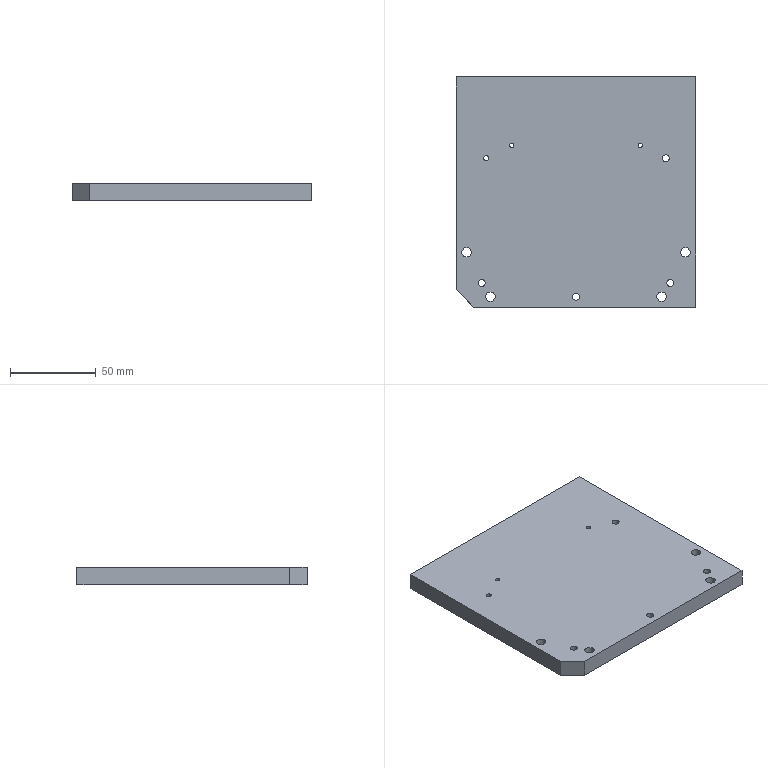Part | 1 solid | 45 faces | box 140 x 134.5 x 10 mm | volume 167544 mm3 | cylinder 23 | plane 22 | commonest cylinder face diameters 10 x10 4 x4 5.5 x4 2.5 x2 10.1 x2 3 x1
STEP:
#1=CARTESIAN_POINT('',(35.,62.25,7.));
#2=VERTEX_POINT('',#1);
#3=CARTESIAN_POINT('',(30.,57.25,7.));
#4=VERTEX_POINT('',#3);
#5=CARTESIAN_POINT('',(30.,62.25,7.));
#6=DIRECTION('',(0.,0.,-1.));
#7=DIRECTION('',(1.,0.,0.));
#8=AXIS2_PLACEMENT_3D('',#5,#6,#7);
#9=CIRCLE('',#8,5.);
#10=EDGE_CURVE('',#2,#4,#9,.T.);
#11=ORIENTED_EDGE('',*,*,#10,.F.);
#12=CARTESIAN_POINT('',(35.,62.25,0.));
#13=VERTEX_POINT('',#12);
#14=CARTESIAN_POINT('',(35.,62.25,7.));
#15=DIRECTION('',(0.,0.,1.));
#16=VECTOR('',#15,1000.);
#17=LINE('',#14,#16);
#18=EDGE_CURVE('',#13,#2,#17,.T.);
#19=ORIENTED_EDGE('',*,*,#18,.F.);
#20=CARTESIAN_POINT('',(30.,57.25,0.));
#21=VERTEX_POINT('',#20);
#22=CARTESIAN_POINT('',(30.,62.25,0.));
#23=DIRECTION('',(0.,0.,1.));
#24=DIRECTION('',(1.,0.,0.));
#25=AXIS2_PLACEMENT_3D('',#22,#23,#24);
#26=CIRCLE('',#25,5.);
#27=EDGE_CURVE('',#21,#13,#26,.T.);
#28=ORIENTED_EDGE('',*,*,#27,.F.);
#29=CARTESIAN_POINT('',(30.,57.25,0.));
#30=DIRECTION('',(0.,0.,-1.));
#31=VECTOR('',#30,1000.);
#32=LINE('',#29,#31);
#33=EDGE_CURVE('',#4,#21,#32,.T.);
#34=ORIENTED_EDGE('',*,*,#33,.F.);
#35=EDGE_LOOP('',(#11,#19,#28,#34));
#36=FACE_BOUND('',#35,.T.);
#37=CARTESIAN_POINT('',(30.,62.25,7.));
#38=DIRECTION('',(0.,0.,1.));
#39=DIRECTION('',(1.,0.,0.));
#40=AXIS2_PLACEMENT_3D('',#37,#38,#39);
#41=CYLINDRICAL_SURFACE('',#40,5.);
#42=ADVANCED_FACE('',(#36),#41,.F.);
#43=CARTESIAN_POINT('',(-30.,57.25,7.));
#44=VERTEX_POINT('',#43);
#45=CARTESIAN_POINT('',(-35.,62.25,7.));
#46=VERTEX_POINT('',#45);
#47=CARTESIAN_POINT('',(-30.,62.25,7.));
#48=DIRECTION('',(0.,0.,-1.));
#49=DIRECTION('',(1.,0.,0.));
#50=AXIS2_PLACEMENT_3D('',#47,#48,#49);
#51=CIRCLE('',#50,5.);
#52=EDGE_CURVE('',#44,#46,#51,.T.);
#53=ORIENTED_EDGE('',*,*,#52,.F.);
#54=CARTESIAN_POINT('',(-30.,57.25,0.));
#55=VERTEX_POINT('',#54);
#56=CARTESIAN_POINT('',(-30.,57.25,7.));
#57=DIRECTION('',(0.,0.,1.));
#58=VECTOR('',#57,1000.);
#59=LINE('',#56,#58);
#60=EDGE_CURVE('',#55,#44,#59,.T.);
#61=ORIENTED_EDGE('',*,*,#60,.F.);
#62=CARTESIAN_POINT('',(-35.,62.25,0.));
#63=VERTEX_POINT('',#62);
#64=CARTESIAN_POINT('',(-30.,62.25,0.));
#65=DIRECTION('',(0.,0.,1.));
#66=DIRECTION('',(1.,0.,0.));
#67=AXIS2_PLACEMENT_3D('',#64,#65,#66);
#68=CIRCLE('',#67,5.);
#69=EDGE_CURVE('',#63,#55,#68,.T.);
#70=ORIENTED_EDGE('',*,*,#69,.F.);
#71=CARTESIAN_POINT('',(-35.,62.25,7.));
#72=DIRECTION('',(0.,0.,-1.));
#73=VECTOR('',#72,1000.);
#74=LINE('',#71,#73);
#75=EDGE_CURVE('',#46,#63,#74,.T.);
#76=ORIENTED_EDGE('',*,*,#75,.F.);
#77=EDGE_LOOP('',(#53,#61,#70,#76));
#78=FACE_BOUND('',#77,.T.);
#79=CARTESIAN_POINT('',(-30.,62.25,7.));
#80=DIRECTION('',(0.,0.,1.));
#81=DIRECTION('',(1.,0.,0.));
#82=AXIS2_PLACEMENT_3D('',#79,#80,#81);
#83=CYLINDRICAL_SURFACE('',#82,5.);
#84=ADVANCED_FACE('',(#78),#83,.F.);
#85=CARTESIAN_POINT('',(30.,-7.75,7.));
#86=VERTEX_POINT('',#85);
#87=CARTESIAN_POINT('',(35.,-12.75,7.));
#88=VERTEX_POINT('',#87);
#89=CARTESIAN_POINT('',(30.,-12.75,7.));
#90=DIRECTION('',(0.,0.,-1.));
#91=DIRECTION('',(1.,0.,0.));
#92=AXIS2_PLACEMENT_3D('',#89,#90,#91);
#93=CIRCLE('',#92,5.);
#94=EDGE_CURVE('',#86,#88,#93,.T.);
#95=ORIENTED_EDGE('',*,*,#94,.F.);
#96=CARTESIAN_POINT('',(30.,-7.75,0.));
#97=VERTEX_POINT('',#96);
#98=CARTESIAN_POINT('',(30.,-7.75,7.));
#99=DIRECTION('',(0.,0.,1.));
#100=VECTOR('',#99,1000.);
#101=LINE('',#98,#100);
#102=EDGE_CURVE('',#97,#86,#101,.T.);
#103=ORIENTED_EDGE('',*,*,#102,.F.);
#104=CARTESIAN_POINT('',(35.,-12.75,0.));
#105=VERTEX_POINT('',#104);
#106=CARTESIAN_POINT('',(30.,-12.75,0.));
#107=DIRECTION('',(0.,0.,1.));
#108=DIRECTION('',(1.,0.,0.));
#109=AXIS2_PLACEMENT_3D('',#106,#107,#108);
#110=CIRCLE('',#109,5.);
#111=EDGE_CURVE('',#105,#97,#110,.T.);
#112=ORIENTED_EDGE('',*,*,#111,.F.);
#113=CARTESIAN_POINT('',(35.,-12.75,0.));
#114=DIRECTION('',(0.,0.,-1.));
#115=VECTOR('',#114,1000.);
#116=LINE('',#113,#115);
#117=EDGE_CURVE('',#88,#105,#116,.T.);
#118=ORIENTED_EDGE('',*,*,#117,.F.);
#119=EDGE_LOOP('',(#95,#103,#112,#118));
#120=FACE_BOUND('',#119,.T.);
#121=CARTESIAN_POINT('',(30.,-12.75,7.));
#122=DIRECTION('',(0.,0.,1.));
#123=DIRECTION('',(1.,0.,0.));
#124=AXIS2_PLACEMENT_3D('',#121,#122,#123);
#125=CYLINDRICAL_SURFACE('',#124,5.);
#126=ADVANCED_FACE('',(#120),#125,.F.);
#127=CARTESIAN_POINT('',(35.,-27.75,7.));
#128=VERTEX_POINT('',#127);
#129=CARTESIAN_POINT('',(30.,-32.75,7.));
#130=VERTEX_POINT('',#129);
#131=CARTESIAN_POINT('',(30.,-27.75,7.));
#132=DIRECTION('',(0.,0.,-1.));
#133=DIRECTION('',(1.,0.,0.));
#134=AXIS2_PLACEMENT_3D('',#131,#132,#133);
#135=CIRCLE('',#134,5.);
#136=EDGE_CURVE('',#128,#130,#135,.T.);
#137=ORIENTED_EDGE('',*,*,#136,.F.);
#138=CARTESIAN_POINT('',(35.,-27.75,0.));
#139=VERTEX_POINT('',#138);
#140=CARTESIAN_POINT('',(35.,-27.75,7.));
#141=DIRECTION('',(0.,0.,1.));
#142=VECTOR('',#141,1000.);
#143=LINE('',#140,#142);
#144=EDGE_CURVE('',#139,#128,#143,.T.);
#145=ORIENTED_EDGE('',*,*,#144,.F.);
#146=CARTESIAN_POINT('',(30.,-32.75,0.));
#147=VERTEX_POINT('',#146);
#148=CARTESIAN_POINT('',(30.,-27.75,0.));
#149=DIRECTION('',(0.,0.,1.));
#150=DIRECTION('',(1.,0.,0.));
#151=AXIS2_PLACEMENT_3D('',#148,#149,#150);
#152=CIRCLE('',#151,5.);
#153=EDGE_CURVE('',#147,#139,#152,.T.);
#154=ORIENTED_EDGE('',*,*,#153,.F.);
#155=CARTESIAN_POINT('',(30.,-32.75,0.));
#156=DIRECTION('',(0.,0.,-1.));
#157=VECTOR('',#156,1000.);
#158=LINE('',#155,#157);
#159=EDGE_CURVE('',#130,#147,#158,.T.);
#160=ORIENTED_EDGE('',*,*,#159,.F.);
#161=EDGE_LOOP('',(#137,#145,#154,#160));
#162=FACE_BOUND('',#161,.T.);
#163=CARTESIAN_POINT('',(30.,-27.75,7.));
#164=DIRECTION('',(0.,0.,1.));
#165=DIRECTION('',(1.,0.,0.));
#166=AXIS2_PLACEMENT_3D('',#163,#164,#165);
#167=CYLINDRICAL_SURFACE('',#166,5.);
#168=ADVANCED_FACE('',(#162),#167,.F.);
#169=CARTESIAN_POINT('',(-35.,-12.75,7.));
#170=VERTEX_POINT('',#169);
#171=CARTESIAN_POINT('',(-30.,-7.75,7.));
#172=VERTEX_POINT('',#171);
#173=CARTESIAN_POINT('',(-30.,-12.75,7.));
#174=DIRECTION('',(0.,0.,-1.));
#175=DIRECTION('',(1.,0.,0.));
#176=AXIS2_PLACEMENT_3D('',#173,#174,#175);
#177=CIRCLE('',#176,5.);
#178=EDGE_CURVE('',#170,#172,#177,.T.);
#179=ORIENTED_EDGE('',*,*,#178,.F.);
#180=CARTESIAN_POINT('',(-35.,-12.75,0.));
#181=VERTEX_POINT('',#180);
#182=CARTESIAN_POINT('',(-35.,-12.75,7.));
#183=DIRECTION('',(0.,0.,1.));
#184=VECTOR('',#183,1000.);
#185=LINE('',#182,#184);
#186=EDGE_CURVE('',#181,#170,#185,.T.);
#187=ORIENTED_EDGE('',*,*,#186,.F.);
#188=CARTESIAN_POINT('',(-30.,-7.75,0.));
#189=VERTEX_POINT('',#188);
#190=CARTESIAN_POINT('',(-30.,-12.75,0.));
#191=DIRECTION('',(0.,0.,1.));
#192=DIRECTION('',(1.,0.,0.));
#193=AXIS2_PLACEMENT_3D('',#190,#191,#192);
#194=CIRCLE('',#193,5.);
#195=EDGE_CURVE('',#189,#181,#194,.T.);
#196=ORIENTED_EDGE('',*,*,#195,.F.);
#197=CARTESIAN_POINT('',(-30.,-7.75,0.));
#198=DIRECTION('',(0.,0.,-1.));
#199=VECTOR('',#198,1000.);
#200=LINE('',#197,#199);
#201=EDGE_CURVE('',#172,#189,#200,.T.);
#202=ORIENTED_EDGE('',*,*,#201,.F.);
#203=EDGE_LOOP('',(#179,#187,#196,#202));
#204=FACE_BOUND('',#203,.T.);
#205=CARTESIAN_POINT('',(-30.,-12.75,7.));
#206=DIRECTION('',(0.,0.,1.));
#207=DIRECTION('',(1.,0.,0.));
#208=AXIS2_PLACEMENT_3D('',#205,#206,#207);
#209=CYLINDRICAL_SURFACE('',#208,5.);
#210=ADVANCED_FACE('',(#204),#209,.F.);
#211=CARTESIAN_POINT('',(-30.,-32.75,7.));
#212=VERTEX_POINT('',#211);
#213=CARTESIAN_POINT('',(-35.,-27.75,7.));
#214=VERTEX_POINT('',#213);
#215=CARTESIAN_POINT('',(-30.,-27.75,7.));
#216=DIRECTION('',(0.,0.,-1.));
#217=DIRECTION('',(1.,0.,0.));
#218=AXIS2_PLACEMENT_3D('',#215,#216,#217);
#219=CIRCLE('',#218,5.);
#220=EDGE_CURVE('',#212,#214,#219,.T.);
#221=ORIENTED_EDGE('',*,*,#220,.F.);
#222=CARTESIAN_POINT('',(-30.,-32.75,0.));
#223=VERTEX_POINT('',#222);
#224=CARTESIAN_POINT('',(-30.,-32.75,7.));
#225=DIRECTION('',(0.,0.,1.));
#226=VECTOR('',#225,1000.);
#227=LINE('',#224,#226);
#228=EDGE_CURVE('',#223,#212,#227,.T.);
#229=ORIENTED_EDGE('',*,*,#228,.F.);
#230=CARTESIAN_POINT('',(-35.,-27.75,0.));
#231=VERTEX_POINT('',#230);
#232=CARTESIAN_POINT('',(-30.,-27.75,0.));
#233=DIRECTION('',(0.,0.,1.));
#234=DIRECTION('',(1.,0.,0.));
#235=AXIS2_PLACEMENT_3D('',#232,#233,#234);
#236=CIRCLE('',#235,5.);
#237=EDGE_CURVE('',#231,#223,#236,.T.);
#238=ORIENTED_EDGE('',*,*,#237,.F.);
#239=CARTESIAN_POINT('',(-35.,-27.75,0.));
#240=DIRECTION('',(0.,0.,-1.));
#241=VECTOR('',#240,1000.);
#242=LINE('',#239,#241);
#243=EDGE_CURVE('',#214,#231,#242,.T.);
#244=ORIENTED_EDGE('',*,*,#243,.F.);
#245=EDGE_LOOP('',(#221,#229,#238,#244));
#246=FACE_BOUND('',#245,.T.);
#247=CARTESIAN_POINT('',(-30.,-27.75,7.));
#248=DIRECTION('',(0.,0.,1.));
#249=DIRECTION('',(1.,0.,0.));
#250=AXIS2_PLACEMENT_3D('',#247,#248,#249);
#251=CYLINDRICAL_SURFACE('',#250,5.);
#252=ADVANCED_FACE('',(#246),#251,.F.);
#253=CARTESIAN_POINT('',(35.,-32.75,7.));
#254=DIRECTION('',(-1.,0.,0.));
#255=VECTOR('',#254,1000.);
#256=LINE('',#253,#255);
#257=EDGE_CURVE('',#130,#212,#256,.T.);
#258=ORIENTED_EDGE('',*,*,#257,.T.);
#259=ORIENTED_EDGE('',*,*,#220,.T.);
#260=CARTESIAN_POINT('',(-35.,-32.75,7.));
#261=DIRECTION('',(0.,1.,0.));
#262=VECTOR('',#261,1000.);
#263=LINE('',#260,#262);
#264=EDGE_CURVE('',#214,#170,#263,.T.);
#265=ORIENTED_EDGE('',*,*,#264,.T.);
#266=ORIENTED_EDGE('',*,*,#178,.T.);
#267=CARTESIAN_POINT('',(35.,-7.75,7.));
#268=DIRECTION('',(1.,0.,0.));
#269=VECTOR('',#268,1000.);
#270=LINE('',#267,#269);
#271=EDGE_CURVE('',#172,#86,#270,.T.);
#272=ORIENTED_EDGE('',*,*,#271,.T.);
#273=ORIENTED_EDGE('',*,*,#94,.T.);
#274=CARTESIAN_POINT('',(35.,-32.75,7.));
#275=DIRECTION('',(0.,-1.,0.));
#276=VECTOR('',#275,1000.);
#277=LINE('',#274,#276);
#278=EDGE_CURVE('',#88,#128,#277,.T.);
#279=ORIENTED_EDGE('',*,*,#278,.T.);
#280=ORIENTED_EDGE('',*,*,#136,.T.);
#281=EDGE_LOOP('',(#258,#259,#265,#266,#272,#273,#279,#280));
#282=FACE_BOUND('',#281,.T.);
#283=CARTESIAN_POINT('',(0.,0.,7.));
#284=DIRECTION('',(0.,0.,1.));
#285=DIRECTION('',(1.,0.,0.));
#286=AXIS2_PLACEMENT_3D('',#283,#284,#285);
#287=PLANE('',#286);
#288=ADVANCED_FACE('',(#282),#287,.F.);
#289=CARTESIAN_POINT('',(35.,-32.75,0.));
#290=DIRECTION('',(-1.,0.,0.));
#291=VECTOR('',#290,1000.);
#292=LINE('',#289,#291);
#293=EDGE_CURVE('',#147,#223,#292,.T.);
#294=ORIENTED_EDGE('',*,*,#293,.T.);
#295=ORIENTED_EDGE('',*,*,#228,.T.);
#296=ORIENTED_EDGE('',*,*,#257,.F.);
#297=ORIENTED_EDGE('',*,*,#159,.T.);
#298=EDGE_LOOP('',(#294,#295,#296,#297));
#299=FACE_BOUND('',#298,.T.);
#300=CARTESIAN_POINT('',(35.,-32.75,7.));
#301=DIRECTION('',(0.,-1.,0.));
#302=DIRECTION('',(0.,0.,-1.));
#303=AXIS2_PLACEMENT_3D('',#300,#301,#302);
#304=PLANE('',#303);
#305=ADVANCED_FACE('',(#299),#304,.F.);
#306=ORIENTED_EDGE('',*,*,#264,.F.);
#307=ORIENTED_EDGE('',*,*,#243,.T.);
#308=CARTESIAN_POINT('',(-35.,-32.75,0.));
#309=DIRECTION('',(0.,1.,0.));
#310=VECTOR('',#309,1000.);
#311=LINE('',#308,#310);
#312=EDGE_CURVE('',#231,#181,#311,.T.);
#313=ORIENTED_EDGE('',*,*,#312,.T.);
#314=ORIENTED_EDGE('',*,*,#186,.T.);
#315=EDGE_LOOP('',(#306,#307,#313,#314));
#316=FACE_BOUND('',#315,.T.);
#317=CARTESIAN_POINT('',(-35.,-32.75,7.));
#318=DIRECTION('',(-1.,0.,0.));
#319=DIRECTION('',(0.,0.,1.));
#320=AXIS2_PLACEMENT_3D('',#317,#318,#319);
#321=PLANE('',#320);
#322=ADVANCED_FACE('',(#316),#321,.F.);
#323=ORIENTED_EDGE('',*,*,#271,.F.);
#324=ORIENTED_EDGE('',*,*,#201,.T.);
#325=CARTESIAN_POINT('',(35.,-7.75,0.));
#326=DIRECTION('',(1.,0.,0.));
#327=VECTOR('',#326,1000.);
#328=LINE('',#325,#327);
#329=EDGE_CURVE('',#189,#97,#328,.T.);
#330=ORIENTED_EDGE('',*,*,#329,.T.);
#331=ORIENTED_EDGE('',*,*,#102,.T.);
#332=EDGE_LOOP('',(#323,#324,#330,#331));
#333=FACE_BOUND('',#332,.T.);
#334=CARTESIAN_POINT('',(35.,-7.75,7.));
#335=DIRECTION('',(0.,1.,0.));
#336=DIRECTION('',(0.,0.,1.));
#337=AXIS2_PLACEMENT_3D('',#334,#335,#336);
#338=PLANE('',#337);
#339=ADVANCED_FACE('',(#333),#338,.F.);
#340=CARTESIAN_POINT('',(35.,-32.75,0.));
#341=DIRECTION('',(0.,-1.,0.));
#342=VECTOR('',#341,1000.);
#343=LINE('',#340,#342);
#344=EDGE_CURVE('',#105,#139,#343,.T.);
#345=ORIENTED_EDGE('',*,*,#344,.T.);
#346=ORIENTED_EDGE('',*,*,#144,.T.);
#347=ORIENTED_EDGE('',*,*,#278,.F.);
#348=ORIENTED_EDGE('',*,*,#117,.T.);
#349=EDGE_LOOP('',(#345,#346,#347,#348));
#350=FACE_BOUND('',#349,.T.);
#351=CARTESIAN_POINT('',(35.,-32.75,7.));
#352=DIRECTION('',(1.,0.,0.));
#353=DIRECTION('',(0.,0.,-1.));
#354=AXIS2_PLACEMENT_3D('',#351,#352,#353);
#355=PLANE('',#354);
#356=ADVANCED_FACE('',(#350),#355,.F.);
#357=CARTESIAN_POINT('',(-35.,57.25,7.));
#358=DIRECTION('',(-1.,0.,0.));
#359=VECTOR('',#358,1000.);
#360=LINE('',#357,#359);
#361=EDGE_CURVE('',#4,#44,#360,.T.);
#362=ORIENTED_EDGE('',*,*,#361,.T.);
#363=ORIENTED_EDGE('',*,*,#52,.T.);
#364=CARTESIAN_POINT('',(-35.,67.25,7.));
#365=VERTEX_POINT('',#364);
#366=CARTESIAN_POINT('',(-35.,0.,7.));
#367=DIRECTION('',(0.,1.,0.));
#368=VECTOR('',#367,1000.);
#369=LINE('',#366,#368);
#370=EDGE_CURVE('',#46,#365,#369,.T.);
#371=ORIENTED_EDGE('',*,*,#370,.T.);
#372=CARTESIAN_POINT('',(35.,67.25,7.));
#373=VERTEX_POINT('',#372);
#374=CARTESIAN_POINT('',(-35.,67.25,7.));
#375=DIRECTION('',(1.,0.,0.));
#376=VECTOR('',#375,1000.);
#377=LINE('',#374,#376);
#378=EDGE_CURVE('',#365,#373,#377,.T.);
#379=ORIENTED_EDGE('',*,*,#378,.T.);
#380=CARTESIAN_POINT('',(35.,0.,7.));
#381=DIRECTION('',(0.,-1.,0.));
#382=VECTOR('',#381,1000.);
#383=LINE('',#380,#382);
#384=EDGE_CURVE('',#373,#2,#383,.T.);
#385=ORIENTED_EDGE('',*,*,#384,.T.);
#386=ORIENTED_EDGE('',*,*,#10,.T.);
#387=EDGE_LOOP('',(#362,#363,#371,#379,#385,#386));
#388=FACE_BOUND('',#387,.T.);
#389=CARTESIAN_POINT('',(0.,0.,7.));
#390=DIRECTION('',(0.,0.,1.));
#391=DIRECTION('',(1.,0.,0.));
#392=AXIS2_PLACEMENT_3D('',#389,#390,#391);
#393=PLANE('',#392);
#394=ADVANCED_FACE('',(#388),#393,.F.);
#395=CARTESIAN_POINT('',(35.,67.25,0.));
#396=VERTEX_POINT('',#395);
#397=CARTESIAN_POINT('',(35.,-32.75,0.));
#398=DIRECTION('',(0.,-1.,0.));
#399=VECTOR('',#398,1000.);
#400=LINE('',#397,#399);
#401=EDGE_CURVE('',#396,#13,#400,.T.);
#402=ORIENTED_EDGE('',*,*,#401,.T.);
#403=ORIENTED_EDGE('',*,*,#18,.T.);
#404=ORIENTED_EDGE('',*,*,#384,.F.);
#405=CARTESIAN_POINT('',(35.,67.25,7.));
#406=DIRECTION('',(0.,0.,-1.));
#407=VECTOR('',#406,1000.);
#408=LINE('',#405,#407);
#409=EDGE_CURVE('',#373,#396,#408,.T.);
#410=ORIENTED_EDGE('',*,*,#409,.T.);
#411=EDGE_LOOP('',(#402,#403,#404,#410));
#412=FACE_BOUND('',#411,.T.);
#413=CARTESIAN_POINT('',(35.,-32.75,7.));
#414=DIRECTION('',(1.,0.,0.));
#415=DIRECTION('',(0.,0.,-1.));
#416=AXIS2_PLACEMENT_3D('',#413,#414,#415);
#417=PLANE('',#416);
#418=ADVANCED_FACE('',(#412),#417,.F.);
#419=CARTESIAN_POINT('',(-35.,57.25,0.));
#420=DIRECTION('',(-1.,0.,0.));
#421=VECTOR('',#420,1000.);
#422=LINE('',#419,#421);
#423=EDGE_CURVE('',#21,#55,#422,.T.);
#424=ORIENTED_EDGE('',*,*,#423,.T.);
#425=ORIENTED_EDGE('',*,*,#60,.T.);
#426=ORIENTED_EDGE('',*,*,#361,.F.);
#427=ORIENTED_EDGE('',*,*,#33,.T.);
#428=EDGE_LOOP('',(#424,#425,#426,#427));
#429=FACE_BOUND('',#428,.T.);
#430=CARTESIAN_POINT('',(-35.,57.25,7.));
#431=DIRECTION('',(0.,-1.,0.));
#432=DIRECTION('',(0.,0.,-1.));
#433=AXIS2_PLACEMENT_3D('',#430,#431,#432);
#434=PLANE('',#433);
#435=ADVANCED_FACE('',(#429),#434,.F.);
#436=ORIENTED_EDGE('',*,*,#370,.F.);
#437=ORIENTED_EDGE('',*,*,#75,.T.);
#438=CARTESIAN_POINT('',(-35.,67.25,0.));
#439=VERTEX_POINT('',#438);
#440=CARTESIAN_POINT('',(-35.,-32.75,0.));
#441=DIRECTION('',(0.,1.,0.));
#442=VECTOR('',#441,1000.);
#443=LINE('',#440,#442);
#444=EDGE_CURVE('',#63,#439,#443,.T.);
#445=ORIENTED_EDGE('',*,*,#444,.T.);
#446=CARTESIAN_POINT('',(-35.,67.25,10.));
#447=DIRECTION('',(0.,0.,-1.));
#448=VECTOR('',#447,1000.);
#449=LINE('',#446,#448);
#450=EDGE_CURVE('',#365,#439,#449,.T.);
#451=ORIENTED_EDGE('',*,*,#450,.F.);
#452=EDGE_LOOP('',(#436,#437,#445,#451));
#453=FACE_BOUND('',#452,.T.);
#454=CARTESIAN_POINT('',(-35.,-32.75,7.));
#455=DIRECTION('',(-1.,0.,0.));
#456=DIRECTION('',(0.,0.,1.));
#457=AXIS2_PLACEMENT_3D('',#454,#455,#456);
#458=PLANE('',#457);
#459=ADVANCED_FACE('',(#453),#458,.F.);
#460=CARTESIAN_POINT('',(32.45,27.25,3.5));
#461=VERTEX_POINT('',#460);
#462=CARTESIAN_POINT('',(37.5,27.25,3.5));
#463=DIRECTION('',(0.,0.,-1.));
#464=DIRECTION('',(-1.,0.,0.));
#465=AXIS2_PLACEMENT_3D('',#462,#463,#464);
#466=CIRCLE('',#465,5.05);
#467=EDGE_CURVE('',#461,#461,#466,.T.);
#468=ORIENTED_EDGE('',*,*,#467,.T.);
#469=EDGE_LOOP('',(#468));
#470=FACE_BOUND('',#469,.T.);
#471=CARTESIAN_POINT('',(36.25,27.25,3.5));
#472=VERTEX_POINT('',#471);
#473=CARTESIAN_POINT('',(37.5,27.25,3.5));
#474=DIRECTION('',(0.,0.,-1.));
#475=DIRECTION('',(-1.,0.,0.));
#476=AXIS2_PLACEMENT_3D('',#473,#474,#475);
#477=CIRCLE('',#476,1.25);
#478=EDGE_CURVE('',#472,#472,#477,.T.);
#479=ORIENTED_EDGE('',*,*,#478,.F.);
#480=EDGE_LOOP('',(#479));
#481=FACE_BOUND('',#480,.T.);
#482=CARTESIAN_POINT('',(37.5,27.25,3.5));
#483=DIRECTION('',(0.,0.,1.));
#484=DIRECTION('',(1.,0.,0.));
#485=AXIS2_PLACEMENT_3D('',#482,#483,#484);
#486=PLANE('',#485);
#487=ADVANCED_FACE('',(#470,#481),#486,.F.);
#488=CARTESIAN_POINT('',(-32.45,27.25,3.5));
#489=VERTEX_POINT('',#488);
#490=CARTESIAN_POINT('',(-37.5,27.25,3.5));
#491=DIRECTION('',(0.,0.,-1.));
#492=DIRECTION('',(1.,0.,0.));
#493=AXIS2_PLACEMENT_3D('',#490,#491,#492);
#494=CIRCLE('',#493,5.05);
#495=EDGE_CURVE('',#489,#489,#494,.T.);
#496=ORIENTED_EDGE('',*,*,#495,.T.);
#497=EDGE_LOOP('',(#496));
#498=FACE_BOUND('',#497,.T.);
#499=CARTESIAN_POINT('',(-36.25,27.25,3.5));
#500=VERTEX_POINT('',#499);
#501=CARTESIAN_POINT('',(-37.5,27.25,3.5));
#502=DIRECTION('',(0.,0.,-1.));
#503=DIRECTION('',(1.,0.,0.));
#504=AXIS2_PLACEMENT_3D('',#501,#502,#503);
#505=CIRCLE('',#504,1.25);
#506=EDGE_CURVE('',#500,#500,#505,.T.);
#507=ORIENTED_EDGE('',*,*,#506,.F.);
#508=EDGE_LOOP('',(#507));
#509=FACE_BOUND('',#508,.T.);
#510=CARTESIAN_POINT('',(37.5,27.25,3.5));
#511=DIRECTION('',(0.,0.,1.));
#512=DIRECTION('',(1.,0.,0.));
#513=AXIS2_PLACEMENT_3D('',#510,#511,#512);
#514=PLANE('',#513);
#515=ADVANCED_FACE('',(#498,#509),#514,.F.);
#516=CARTESIAN_POINT('',(-70.,-57.25,10.));
#517=VERTEX_POINT('',#516);
#518=CARTESIAN_POINT('',(-60.,-67.25,10.));
#519=VERTEX_POINT('',#518);
#520=CARTESIAN_POINT('',(-63.625,-63.625,10.));
#521=DIRECTION('',(0.7071,-0.7071,0.));
#522=VECTOR('',#521,1000.);
#523=LINE('',#520,#522);
#524=EDGE_CURVE('',#517,#519,#523,.T.);
#525=ORIENTED_EDGE('',*,*,#524,.F.);
#526=CARTESIAN_POINT('',(-70.,-57.25,0.));
#527=VERTEX_POINT('',#526);
#528=CARTESIAN_POINT('',(-70.,-57.25,10.));
#529=DIRECTION('',(0.,0.,1.));
#530=VECTOR('',#529,1000.);
#531=LINE('',#528,#530);
#532=EDGE_CURVE('',#527,#517,#531,.T.);
#533=ORIENTED_EDGE('',*,*,#532,.F.);
#534=CARTESIAN_POINT('',(-60.,-67.25,0.));
#535=VERTEX_POINT('',#534);
#536=CARTESIAN_POINT('',(-60.,-67.25,0.));
#537=DIRECTION('',(-0.7071,0.7071,0.));
#538=VECTOR('',#537,1000.);
#539=LINE('',#536,#538);
#540=EDGE_CURVE('',#535,#527,#539,.T.);
#541=ORIENTED_EDGE('',*,*,#540,.F.);
#542=CARTESIAN_POINT('',(-60.,-67.25,10.));
#543=DIRECTION('',(0.,0.,-1.));
#544=VECTOR('',#543,1000.);
#545=LINE('',#542,#544);
#546=EDGE_CURVE('',#519,#535,#545,.T.);
#547=ORIENTED_EDGE('',*,*,#546,.F.);
#548=EDGE_LOOP('',(#525,#533,#541,#547));
#549=FACE_BOUND('',#548,.T.);
#550=CARTESIAN_POINT('',(-60.,-67.25,10.));
#551=DIRECTION('',(0.7071,0.7071,0.));
#552=DIRECTION('',(0.,0.,-1.));
#553=AXIS2_PLACEMENT_3D('',#550,#551,#552);
#554=PLANE('',#553);
#555=ADVANCED_FACE('',(#549),#554,.F.);
#556=CARTESIAN_POINT('',(45.,-61.25,5.4));
#557=VERTEX_POINT('',#556);
#558=CARTESIAN_POINT('',(50.,-61.25,5.4));
#559=DIRECTION('',(0.,0.,-1.));
#560=DIRECTION('',(-1.,0.,0.));
#561=AXIS2_PLACEMENT_3D('',#558,#559,#560);
#562=CIRCLE('',#561,5.);
#563=EDGE_CURVE('',#557,#557,#562,.T.);
#564=ORIENTED_EDGE('',*,*,#563,.T.);
#565=EDGE_LOOP('',(#564));
#566=FACE_BOUND('',#565,.T.);
#567=CARTESIAN_POINT('',(47.25,-61.25,5.4));
#568=VERTEX_POINT('',#567);
#569=CARTESIAN_POINT('',(50.,-61.25,5.4));
#570=DIRECTION('',(0.,0.,-1.));
#571=DIRECTION('',(-1.,0.,0.));
#572=AXIS2_PLACEMENT_3D('',#569,#570,#571);
#573=CIRCLE('',#572,2.75);
#574=EDGE_CURVE('',#568,#568,#573,.T.);
#575=ORIENTED_EDGE('',*,*,#574,.F.);
#576=EDGE_LOOP('',(#575));
#577=FACE_BOUND('',#576,.T.);
#578=CARTESIAN_POINT('',(52.75,-61.25,5.4));
#579=DIRECTION('',(0.,0.,1.));
#580=DIRECTION('',(1.,0.,0.));
#581=AXIS2_PLACEMENT_3D('',#578,#579,#580);
#582=PLANE('',#581);
#583=ADVANCED_FACE('',(#566,#577),#582,.F.);
#584=CARTESIAN_POINT('',(-45.,-61.25,5.4));
#585=VERTEX_POINT('',#584);
#586=CARTESIAN_POINT('',(-50.,-61.25,5.4));
#587=DIRECTION('',(0.,0.,-1.));
#588=DIRECTION('',(1.,0.,0.));
#589=AXIS2_PLACEMENT_3D('',#586,#587,#588);
#590=CIRCLE('',#589,5.);
#591=EDGE_CURVE('',#585,#585,#590,.T.);
#592=ORIENTED_EDGE('',*,*,#591,.T.);
#593=EDGE_LOOP('',(#592));
#594=FACE_BOUND('',#593,.T.);
#595=CARTESIAN_POINT('',(-47.25,-61.25,5.4));
#596=VERTEX_POINT('',#595);
#597=CARTESIAN_POINT('',(-50.,-61.25,5.4));
#598=DIRECTION('',(0.,0.,-1.));
#599=DIRECTION('',(1.,0.,0.));
#600=AXIS2_PLACEMENT_3D('',#597,#598,#599);
#601=CIRCLE('',#600,2.75);
#602=EDGE_CURVE('',#596,#596,#601,.T.);
#603=ORIENTED_EDGE('',*,*,#602,.F.);
#604=EDGE_LOOP('',(#603));
#605=FACE_BOUND('',#604,.T.);
#606=CARTESIAN_POINT('',(52.75,-61.25,5.4));
#607=DIRECTION('',(0.,0.,1.));
#608=DIRECTION('',(1.,0.,0.));
#609=AXIS2_PLACEMENT_3D('',#606,#607,#608);
#610=PLANE('',#609);
#611=ADVANCED_FACE('',(#594,#605),#610,.F.);
#612=CARTESIAN_POINT('',(69.,-35.25,5.4));
#613=VERTEX_POINT('',#612);
#614=CARTESIAN_POINT('',(64.,-35.25,5.4));
#615=DIRECTION('',(0.,0.,-1.));
#616=DIRECTION('',(1.,0.,0.));
#617=AXIS2_PLACEMENT_3D('',#614,#615,#616);
#618=CIRCLE('',#617,5.);
#619=EDGE_CURVE('',#613,#613,#618,.T.);
#620=ORIENTED_EDGE('',*,*,#619,.T.);
#621=EDGE_LOOP('',(#620));
#622=FACE_BOUND('',#621,.T.);
#623=CARTESIAN_POINT('',(66.75,-35.25,5.4));
#624=VERTEX_POINT('',#623);
#625=CARTESIAN_POINT('',(64.,-35.25,5.4));
#626=DIRECTION('',(0.,0.,-1.));
#627=DIRECTION('',(1.,0.,0.));
#628=AXIS2_PLACEMENT_3D('',#625,#626,#627);
#629=CIRCLE('',#628,2.75);
#630=EDGE_CURVE('',#624,#624,#629,.T.);
#631=ORIENTED_EDGE('',*,*,#630,.F.);
#632=EDGE_LOOP('',(#631));
#633=FACE_BOUND('',#632,.T.);
#634=CARTESIAN_POINT('',(52.75,-61.25,5.4));
#635=DIRECTION('',(0.,0.,1.));
#636=DIRECTION('',(1.,0.,0.));
#637=AXIS2_PLACEMENT_3D('',#634,#635,#636);
#638=PLANE('',#637);
#639=ADVANCED_FACE('',(#622,#633),#638,.F.);
#640=CARTESIAN_POINT('',(-59.,-35.25,5.4));
#641=VERTEX_POINT('',#640);
#642=CARTESIAN_POINT('',(-64.,-35.25,5.4));
#643=DIRECTION('',(0.,0.,-1.));
#644=DIRECTION('',(1.,0.,0.));
#645=AXIS2_PLACEMENT_3D('',#642,#643,#644);
#646=CIRCLE('',#645,5.);
#647=EDGE_CURVE('',#641,#641,#646,.T.);
#648=ORIENTED_EDGE('',*,*,#647,.T.);
#649=EDGE_LOOP('',(#648));
#650=FACE_BOUND('',#649,.T.);
#651=CARTESIAN_POINT('',(-61.25,-35.25,5.4));
#652=VERTEX_POINT('',#651);
#653=CARTESIAN_POINT('',(-64.,-35.25,5.4));
#654=DIRECTION('',(0.,0.,-1.));
#655=DIRECTION('',(1.,0.,0.));
#656=AXIS2_PLACEMENT_3D('',#653,#654,#655);
#657=CIRCLE('',#656,2.75);
#658=EDGE_CURVE('',#652,#652,#657,.T.);
#659=ORIENTED_EDGE('',*,*,#658,.F.);
#660=EDGE_LOOP('',(#659));
#661=FACE_BOUND('',#660,.T.);
#662=CARTESIAN_POINT('',(52.75,-61.25,5.4));
#663=DIRECTION('',(0.,0.,1.));
#664=DIRECTION('',(1.,0.,0.));
#665=AXIS2_PLACEMENT_3D('',#662,#663,#664);
#666=PLANE('',#665);
#667=ADVANCED_FACE('',(#650,#661),#666,.F.);
#668=CARTESIAN_POINT('',(-70.,67.25,10.));
#669=VERTEX_POINT('',#668);
#670=CARTESIAN_POINT('',(-70.,67.25,10.));
#671=DIRECTION('',(0.,-1.,0.));
#672=VECTOR('',#671,1000.);
#673=LINE('',#670,#672);
#674=EDGE_CURVE('',#669,#517,#673,.T.);
#675=ORIENTED_EDGE('',*,*,#674,.T.);
#676=ORIENTED_EDGE('',*,*,#524,.T.);
#677=CARTESIAN_POINT('',(70.,-67.25,10.));
#678=VERTEX_POINT('',#677);
#679=CARTESIAN_POINT('',(-70.,-67.25,10.));
#680=DIRECTION('',(1.,0.,0.));
#681=VECTOR('',#680,1000.);
#682=LINE('',#679,#681);
#683=EDGE_CURVE('',#519,#678,#682,.T.);
#684=ORIENTED_EDGE('',*,*,#683,.T.);
#685=CARTESIAN_POINT('',(70.,67.25,10.));
#686=VERTEX_POINT('',#685);
#687=CARTESIAN_POINT('',(70.,67.25,10.));
#688=DIRECTION('',(0.,1.,0.));
#689=VECTOR('',#688,1000.);
#690=LINE('',#687,#689);
#691=EDGE_CURVE('',#678,#686,#690,.T.);
#692=ORIENTED_EDGE('',*,*,#691,.T.);
#693=CARTESIAN_POINT('',(-70.,67.25,10.));
#694=DIRECTION('',(-1.,0.,0.));
#695=VECTOR('',#694,1000.);
#696=LINE('',#693,#695);
#697=EDGE_CURVE('',#686,#669,#696,.T.);
#698=ORIENTED_EDGE('',*,*,#697,.T.);
#699=EDGE_LOOP('',(#675,#676,#684,#692,#698));
#700=FACE_BOUND('',#699,.T.);
#701=CARTESIAN_POINT('',(-66.75,-35.25,10.));
#702=VERTEX_POINT('',#701);
#703=CARTESIAN_POINT('',(-64.,-35.25,10.));
#704=DIRECTION('',(0.,0.,-1.));
#705=DIRECTION('',(-1.,0.,0.));
#706=AXIS2_PLACEMENT_3D('',#703,#704,#705);
#707=CIRCLE('',#706,2.75);
#708=EDGE_CURVE('',#702,#702,#707,.T.);
#709=ORIENTED_EDGE('',*,*,#708,.T.);
#710=EDGE_LOOP('',(#709));
#711=FACE_BOUND('',#710,.T.);
#712=CARTESIAN_POINT('',(61.25,-35.25,10.));
#713=VERTEX_POINT('',#712);
#714=CARTESIAN_POINT('',(64.,-35.25,10.));
#715=DIRECTION('',(0.,0.,-1.));
#716=DIRECTION('',(-1.,0.,0.));
#717=AXIS2_PLACEMENT_3D('',#714,#715,#716);
#718=CIRCLE('',#717,2.75);
#719=EDGE_CURVE('',#713,#713,#718,.T.);
#720=ORIENTED_EDGE('',*,*,#719,.T.);
#721=EDGE_LOOP('',(#720));
#722=FACE_BOUND('',#721,.T.);
#723=CARTESIAN_POINT('',(-52.75,-61.25,10.));
#724=VERTEX_POINT('',#723);
#725=CARTESIAN_POINT('',(-50.,-61.25,10.));
#726=DIRECTION('',(0.,0.,-1.));
#727=DIRECTION('',(-1.,0.,0.));
#728=AXIS2_PLACEMENT_3D('',#725,#726,#727);
#729=CIRCLE('',#728,2.75);
#730=EDGE_CURVE('',#724,#724,#729,.T.);
#731=ORIENTED_EDGE('',*,*,#730,.T.);
#732=EDGE_LOOP('',(#731));
#733=FACE_BOUND('',#732,.T.);
#734=CARTESIAN_POINT('',(47.25,-61.25,10.));
#735=VERTEX_POINT('',#734);
#736=CARTESIAN_POINT('',(50.,-61.25,10.));
#737=DIRECTION('',(0.,0.,-1.));
#738=DIRECTION('',(-1.,0.,0.));
#739=AXIS2_PLACEMENT_3D('',#736,#737,#738);
#740=CIRCLE('',#739,2.75);
#741=EDGE_CURVE('',#735,#735,#740,.T.);
#742=ORIENTED_EDGE('',*,*,#741,.T.);
#743=EDGE_LOOP('',(#742));
#744=FACE_BOUND('',#743,.T.);
#745=CARTESIAN_POINT('',(-57.,-53.25,10.));
#746=VERTEX_POINT('',#745);
#747=CARTESIAN_POINT('',(-55.,-53.25,10.));
#748=DIRECTION('',(0.,0.,-1.));
#749=DIRECTION('',(-1.,0.,0.));
#750=AXIS2_PLACEMENT_3D('',#747,#748,#749);
#751=CIRCLE('',#750,2.);
#752=EDGE_CURVE('',#746,#746,#751,.T.);
#753=ORIENTED_EDGE('',*,*,#752,.T.);
#754=EDGE_LOOP('',(#753));
#755=FACE_BOUND('',#754,.T.);
#756=CARTESIAN_POINT('',(53.,-53.25,10.));
#757=VERTEX_POINT('',#756);
#758=CARTESIAN_POINT('',(55.,-53.25,10.));
#759=DIRECTION('',(0.,0.,-1.));
#760=DIRECTION('',(-1.,0.,0.));
#761=AXIS2_PLACEMENT_3D('',#758,#759,#760);
#762=CIRCLE('',#761,2.);
#763=EDGE_CURVE('',#757,#757,#762,.T.);
#764=ORIENTED_EDGE('',*,*,#763,.T.);
#765=EDGE_LOOP('',(#764));
#766=FACE_BOUND('',#765,.T.);
#767=CARTESIAN_POINT('',(-2.,-61.25,10.));
#768=VERTEX_POINT('',#767);
#769=CARTESIAN_POINT('',(0.,-61.25,10.));
#770=DIRECTION('',(0.,0.,-1.));
#771=DIRECTION('',(-1.,0.,0.));
#772=AXIS2_PLACEMENT_3D('',#769,#770,#771);
#773=CIRCLE('',#772,2.);
#774=EDGE_CURVE('',#768,#768,#773,.T.);
#775=ORIENTED_EDGE('',*,*,#774,.T.);
#776=EDGE_LOOP('',(#775));
#777=FACE_BOUND('',#776,.T.);
#778=CARTESIAN_POINT('',(50.5,19.75,10.));
#779=VERTEX_POINT('',#778);
#780=CARTESIAN_POINT('',(52.5,19.75,10.));
#781=DIRECTION('',(0.,0.,-1.));
#782=DIRECTION('',(-1.,0.,0.));
#783=AXIS2_PLACEMENT_3D('',#780,#781,#782);
#784=CIRCLE('',#783,2.);
#785=EDGE_CURVE('',#779,#779,#784,.T.);
#786=ORIENTED_EDGE('',*,*,#785,.T.);
#787=EDGE_LOOP('',(#786));
#788=FACE_BOUND('',#787,.T.);
#789=CARTESIAN_POINT('',(-54.,19.75,10.));
#790=VERTEX_POINT('',#789);
#791=CARTESIAN_POINT('',(-52.5,19.75,10.));
#792=DIRECTION('',(0.,0.,-1.));
#793=DIRECTION('',(-1.,0.,0.));
#794=AXIS2_PLACEMENT_3D('',#791,#792,#793);
#795=CIRCLE('',#794,1.5);
#796=EDGE_CURVE('',#790,#790,#795,.T.);
#797=ORIENTED_EDGE('',*,*,#796,.T.);
#798=EDGE_LOOP('',(#797));
#799=FACE_BOUND('',#798,.T.);
#800=CARTESIAN_POINT('',(-38.75,27.25,10.));
#801=VERTEX_POINT('',#800);
#802=CARTESIAN_POINT('',(-37.5,27.25,10.));
#803=DIRECTION('',(0.,0.,-1.));
#804=DIRECTION('',(-1.,0.,0.));
#805=AXIS2_PLACEMENT_3D('',#802,#803,#804);
#806=CIRCLE('',#805,1.25);
#807=EDGE_CURVE('',#801,#801,#806,.T.);
#808=ORIENTED_EDGE('',*,*,#807,.T.);
#809=EDGE_LOOP('',(#808));
#810=FACE_BOUND('',#809,.T.);
#811=CARTESIAN_POINT('',(36.25,27.25,10.));
#812=VERTEX_POINT('',#811);
#813=CARTESIAN_POINT('',(37.5,27.25,10.));
#814=DIRECTION('',(0.,0.,-1.));
#815=DIRECTION('',(-1.,0.,0.));
#816=AXIS2_PLACEMENT_3D('',#813,#814,#815);
#817=CIRCLE('',#816,1.25);
#818=EDGE_CURVE('',#812,#812,#817,.T.);
#819=ORIENTED_EDGE('',*,*,#818,.T.);
#820=EDGE_LOOP('',(#819));
#821=FACE_BOUND('',#820,.T.);
#822=CARTESIAN_POINT('',(0.,0.,10.));
#823=DIRECTION('',(0.,0.,1.));
#824=DIRECTION('',(1.,0.,0.));
#825=AXIS2_PLACEMENT_3D('',#822,#823,#824);
#826=PLANE('',#825);
#827=ADVANCED_FACE('',(#700,#711,#722,#733,#744,#755,#766,#777,#788,#799,#810,#821),#826,.T.);
#828=ORIENTED_EDGE('',*,*,#683,.F.);
#829=ORIENTED_EDGE('',*,*,#546,.T.);
#830=CARTESIAN_POINT('',(70.,-67.25,0.));
#831=VERTEX_POINT('',#830);
#832=CARTESIAN_POINT('',(-70.,-67.25,0.));
#833=DIRECTION('',(1.,0.,0.));
#834=VECTOR('',#833,1000.);
#835=LINE('',#832,#834);
#836=EDGE_CURVE('',#535,#831,#835,.T.);
#837=ORIENTED_EDGE('',*,*,#836,.T.);
#838=CARTESIAN_POINT('',(70.,-67.25,10.));
#839=DIRECTION('',(0.,0.,-1.));
#840=VECTOR('',#839,1000.);
#841=LINE('',#838,#840);
#842=EDGE_CURVE('',#678,#831,#841,.T.);
#843=ORIENTED_EDGE('',*,*,#842,.F.);
#844=EDGE_LOOP('',(#828,#829,#837,#843));
#845=FACE_BOUND('',#844,.T.);
#846=CARTESIAN_POINT('',(-70.,-67.25,10.));
#847=DIRECTION('',(0.,1.,0.));
#848=DIRECTION('',(0.,0.,1.));
#849=AXIS2_PLACEMENT_3D('',#846,#847,#848);
#850=PLANE('',#849);
#851=ADVANCED_FACE('',(#845),#850,.F.);
#852=CARTESIAN_POINT('',(-70.,67.25,0.));
#853=VERTEX_POINT('',#852);
#854=CARTESIAN_POINT('',(-70.,67.25,0.));
#855=DIRECTION('',(0.,-1.,0.));
#856=VECTOR('',#855,1000.);
#857=LINE('',#854,#856);
#858=EDGE_CURVE('',#853,#527,#857,.T.);
#859=ORIENTED_EDGE('',*,*,#858,.T.);
#860=ORIENTED_EDGE('',*,*,#532,.T.);
#861=ORIENTED_EDGE('',*,*,#674,.F.);
#862=CARTESIAN_POINT('',(-70.,67.25,10.));
#863=DIRECTION('',(0.,0.,-1.));
#864=VECTOR('',#863,1000.);
#865=LINE('',#862,#864);
#866=EDGE_CURVE('',#669,#853,#865,.T.);
#867=ORIENTED_EDGE('',*,*,#866,.T.);
#868=EDGE_LOOP('',(#859,#860,#861,#867));
#869=FACE_BOUND('',#868,.T.);
#870=CARTESIAN_POINT('',(-70.,67.25,10.));
#871=DIRECTION('',(1.,0.,0.));
#872=DIRECTION('',(0.,1.,0.));
#873=AXIS2_PLACEMENT_3D('',#870,#871,#872);
#874=PLANE('',#873);
#875=ADVANCED_FACE('',(#869),#874,.F.);
#876=ORIENTED_EDGE('',*,*,#378,.F.);
#877=ORIENTED_EDGE('',*,*,#450,.T.);
#878=CARTESIAN_POINT('',(-70.,67.25,0.));
#879=DIRECTION('',(-1.,0.,0.));
#880=VECTOR('',#879,1000.);
#881=LINE('',#878,#880);
#882=EDGE_CURVE('',#439,#853,#881,.T.);
#883=ORIENTED_EDGE('',*,*,#882,.T.);
#884=ORIENTED_EDGE('',*,*,#866,.F.);
#885=ORIENTED_EDGE('',*,*,#697,.F.);
#886=CARTESIAN_POINT('',(70.,67.25,0.));
#887=VERTEX_POINT('',#886);
#888=CARTESIAN_POINT('',(70.,67.25,10.));
#889=DIRECTION('',(0.,0.,-1.));
#890=VECTOR('',#889,1000.);
#891=LINE('',#888,#890);
#892=EDGE_CURVE('',#686,#887,#891,.T.);
#893=ORIENTED_EDGE('',*,*,#892,.T.);
#894=CARTESIAN_POINT('',(-70.,67.25,0.));
#895=DIRECTION('',(-1.,0.,0.));
#896=VECTOR('',#895,1000.);
#897=LINE('',#894,#896);
#898=EDGE_CURVE('',#887,#396,#897,.T.);
#899=ORIENTED_EDGE('',*,*,#898,.T.);
#900=ORIENTED_EDGE('',*,*,#409,.F.);
#901=EDGE_LOOP('',(#876,#877,#883,#884,#885,#893,#899,#900));
#902=FACE_BOUND('',#901,.T.);
#903=CARTESIAN_POINT('',(-70.,67.25,10.));
#904=DIRECTION('',(0.,-1.,0.));
#905=DIRECTION('',(1.,0.,0.));
#906=AXIS2_PLACEMENT_3D('',#903,#904,#905);
#907=PLANE('',#906);
#908=ADVANCED_FACE('',(#902),#907,.F.);
#909=CARTESIAN_POINT('',(70.,67.25,0.));
#910=DIRECTION('',(0.,1.,0.));
#911=VECTOR('',#910,1000.);
#912=LINE('',#909,#911);
#913=EDGE_CURVE('',#831,#887,#912,.T.);
#914=ORIENTED_EDGE('',*,*,#913,.T.);
#915=ORIENTED_EDGE('',*,*,#892,.F.);
#916=ORIENTED_EDGE('',*,*,#691,.F.);
#917=ORIENTED_EDGE('',*,*,#842,.T.);
#918=EDGE_LOOP('',(#914,#915,#916,#917));
#919=FACE_BOUND('',#918,.T.);
#920=CARTESIAN_POINT('',(70.,67.25,10.));
#921=DIRECTION('',(-1.,0.,0.));
#922=DIRECTION('',(0.,-1.,0.));
#923=AXIS2_PLACEMENT_3D('',#920,#921,#922);
#924=PLANE('',#923);
#925=ADVANCED_FACE('',(#919),#924,.F.);
#926=CARTESIAN_POINT('',(32.45,27.25,0.));
#927=VERTEX_POINT('',#926);
#928=CARTESIAN_POINT('',(37.5,27.25,0.));
#929=DIRECTION('',(0.,0.,-1.));
#930=DIRECTION('',(-1.,0.,0.));
#931=AXIS2_PLACEMENT_3D('',#928,#929,#930);
#932=CIRCLE('',#931,5.05);
#933=EDGE_CURVE('',#927,#927,#932,.T.);
#934=ORIENTED_EDGE('',*,*,#933,.F.);
#935=EDGE_LOOP('',(#934));
#936=FACE_BOUND('',#935,.T.);
#937=ORIENTED_EDGE('',*,*,#882,.F.);
#938=ORIENTED_EDGE('',*,*,#444,.F.);
#939=ORIENTED_EDGE('',*,*,#69,.T.);
#940=ORIENTED_EDGE('',*,*,#423,.F.);
#941=ORIENTED_EDGE('',*,*,#27,.T.);
#942=ORIENTED_EDGE('',*,*,#401,.F.);
#943=ORIENTED_EDGE('',*,*,#898,.F.);
#944=ORIENTED_EDGE('',*,*,#913,.F.);
#945=ORIENTED_EDGE('',*,*,#836,.F.);
#946=ORIENTED_EDGE('',*,*,#540,.T.);
#947=ORIENTED_EDGE('',*,*,#858,.F.);
#948=EDGE_LOOP('',(#937,#938,#939,#940,#941,#942,#943,#944,#945,#946,#947));
#949=FACE_BOUND('',#948,.T.);
#950=CARTESIAN_POINT('',(-69.,-35.25,0.));
#951=VERTEX_POINT('',#950);
#952=CARTESIAN_POINT('',(-64.,-35.25,0.));
#953=DIRECTION('',(0.,0.,-1.));
#954=DIRECTION('',(-1.,0.,0.));
#955=AXIS2_PLACEMENT_3D('',#952,#953,#954);
#956=CIRCLE('',#955,5.);
#957=EDGE_CURVE('',#951,#951,#956,.T.);
#958=ORIENTED_EDGE('',*,*,#957,.F.);
#959=EDGE_LOOP('',(#958));
#960=FACE_BOUND('',#959,.T.);
#961=CARTESIAN_POINT('',(59.,-35.25,0.));
#962=VERTEX_POINT('',#961);
#963=CARTESIAN_POINT('',(64.,-35.25,0.));
#964=DIRECTION('',(0.,0.,-1.));
#965=DIRECTION('',(-1.,0.,0.));
#966=AXIS2_PLACEMENT_3D('',#963,#964,#965);
#967=CIRCLE('',#966,5.);
#968=EDGE_CURVE('',#962,#962,#967,.T.);
#969=ORIENTED_EDGE('',*,*,#968,.F.);
#970=EDGE_LOOP('',(#969));
#971=FACE_BOUND('',#970,.T.);
#972=CARTESIAN_POINT('',(-55.,-61.25,0.));
#973=VERTEX_POINT('',#972);
#974=CARTESIAN_POINT('',(-50.,-61.25,0.));
#975=DIRECTION('',(0.,0.,-1.));
#976=DIRECTION('',(-1.,0.,0.));
#977=AXIS2_PLACEMENT_3D('',#974,#975,#976);
#978=CIRCLE('',#977,5.);
#979=EDGE_CURVE('',#973,#973,#978,.T.);
#980=ORIENTED_EDGE('',*,*,#979,.F.);
#981=EDGE_LOOP('',(#980));
#982=FACE_BOUND('',#981,.T.);
#983=CARTESIAN_POINT('',(45.,-61.25,0.));
#984=VERTEX_POINT('',#983);
#985=CARTESIAN_POINT('',(50.,-61.25,0.));
#986=DIRECTION('',(0.,0.,-1.));
#987=DIRECTION('',(-1.,0.,0.));
#988=AXIS2_PLACEMENT_3D('',#985,#986,#987);
#989=CIRCLE('',#988,5.);
#990=EDGE_CURVE('',#984,#984,#989,.T.);
#991=ORIENTED_EDGE('',*,*,#990,.F.);
#992=EDGE_LOOP('',(#991));
#993=FACE_BOUND('',#992,.T.);
#994=CARTESIAN_POINT('',(-57.,-53.25,0.));
#995=VERTEX_POINT('',#994);
#996=CARTESIAN_POINT('',(-55.,-53.25,0.));
#997=DIRECTION('',(0.,0.,-1.));
#998=DIRECTION('',(-1.,0.,0.));
#999=AXIS2_PLACEMENT_3D('',#996,#997,#998);
#1000=CIRCLE('',#999,2.);
#1001=EDGE_CURVE('',#995,#995,#1000,.T.);
#1002=ORIENTED_EDGE('',*,*,#1001,.F.);
#1003=EDGE_LOOP('',(#1002));
#1004=FACE_BOUND('',#1003,.T.);
#1005=CARTESIAN_POINT('',(53.,-53.25,0.));
#1006=VERTEX_POINT('',#1005);
#1007=CARTESIAN_POINT('',(55.,-53.25,0.));
#1008=DIRECTION('',(0.,0.,-1.));
#1009=DIRECTION('',(-1.,0.,0.));
#1010=AXIS2_PLACEMENT_3D('',#1007,#1008,#1009);
#1011=CIRCLE('',#1010,2.);
#1012=EDGE_CURVE('',#1006,#1006,#1011,.T.);
#1013=ORIENTED_EDGE('',*,*,#1012,.F.);
#1014=EDGE_LOOP('',(#1013));
#1015=FACE_BOUND('',#1014,.T.);
#1016=CARTESIAN_POINT('',(-2.,-61.25,0.));
#1017=VERTEX_POINT('',#1016);
#1018=CARTESIAN_POINT('',(0.,-61.25,0.));
#1019=DIRECTION('',(0.,0.,-1.));
#1020=DIRECTION('',(-1.,0.,0.));
#1021=AXIS2_PLACEMENT_3D('',#1018,#1019,#1020);
#1022=CIRCLE('',#1021,2.);
#1023=EDGE_CURVE('',#1017,#1017,#1022,.T.);
#1024=ORIENTED_EDGE('',*,*,#1023,.F.);
#1025=EDGE_LOOP('',(#1024));
#1026=FACE_BOUND('',#1025,.T.);
#1027=CARTESIAN_POINT('',(50.5,19.75,0.));
#1028=VERTEX_POINT('',#1027);
#1029=CARTESIAN_POINT('',(52.5,19.75,0.));
#1030=DIRECTION('',(0.,0.,-1.));
#1031=DIRECTION('',(-1.,0.,0.));
#1032=AXIS2_PLACEMENT_3D('',#1029,#1030,#1031);
#1033=CIRCLE('',#1032,2.);
#1034=EDGE_CURVE('',#1028,#1028,#1033,.T.);
#1035=ORIENTED_EDGE('',*,*,#1034,.F.);
#1036=EDGE_LOOP('',(#1035));
#1037=FACE_BOUND('',#1036,.T.);
#1038=CARTESIAN_POINT('',(-54.,19.75,0.));
#1039=VERTEX_POINT('',#1038);
#1040=CARTESIAN_POINT('',(-52.5,19.75,0.));
#1041=DIRECTION('',(0.,0.,-1.));
#1042=DIRECTION('',(-1.,0.,0.));
#1043=AXIS2_PLACEMENT_3D('',#1040,#1041,#1042);
#1044=CIRCLE('',#1043,1.5);
#1045=EDGE_CURVE('',#1039,#1039,#1044,.T.);
#1046=ORIENTED_EDGE('',*,*,#1045,.F.);
#1047=EDGE_LOOP('',(#1046));
#1048=FACE_BOUND('',#1047,.T.);
#1049=CARTESIAN_POINT('',(-42.55,27.25,0.));
#1050=VERTEX_POINT('',#1049);
#1051=CARTESIAN_POINT('',(-37.5,27.25,0.));
#1052=DIRECTION('',(0.,0.,-1.));
#1053=DIRECTION('',(-1.,0.,0.));
#1054=AXIS2_PLACEMENT_3D('',#1051,#1052,#1053);
#1055=CIRCLE('',#1054,5.05);
#1056=EDGE_CURVE('',#1050,#1050,#1055,.T.);
#1057=ORIENTED_EDGE('',*,*,#1056,.F.);
#1058=EDGE_LOOP('',(#1057));
#1059=FACE_BOUND('',#1058,.T.);
#1060=ORIENTED_EDGE('',*,*,#293,.F.);
#1061=ORIENTED_EDGE('',*,*,#153,.T.);
#1062=ORIENTED_EDGE('',*,*,#344,.F.);
#1063=ORIENTED_EDGE('',*,*,#111,.T.);
#1064=ORIENTED_EDGE('',*,*,#329,.F.);
#1065=ORIENTED_EDGE('',*,*,#195,.T.);
#1066=ORIENTED_EDGE('',*,*,#312,.F.);
#1067=ORIENTED_EDGE('',*,*,#237,.T.);
#1068=EDGE_LOOP('',(#1060,#1061,#1062,#1063,#1064,#1065,#1066,#1067));
#1069=FACE_BOUND('',#1068,.T.);
#1070=CARTESIAN_POINT('',(0.,0.,0.));
#1071=DIRECTION('',(0.,0.,1.));
#1072=DIRECTION('',(1.,0.,0.));
#1073=AXIS2_PLACEMENT_3D('',#1070,#1071,#1072);
#1074=PLANE('',#1073);
#1075=ADVANCED_FACE('',(#936,#949,#960,#971,#982,#993,#1004,#1015,#1026,#1037,#1048,#1059,#1069),#1074,.F.);
#1076=ORIENTED_EDGE('',*,*,#658,.T.);
#1077=EDGE_LOOP('',(#1076));
#1078=FACE_BOUND('',#1077,.T.);
#1079=ORIENTED_EDGE('',*,*,#708,.F.);
#1080=EDGE_LOOP('',(#1079));
#1081=FACE_BOUND('',#1080,.T.);
#1082=CARTESIAN_POINT('',(-64.,-35.25,0.));
#1083=DIRECTION('',(0.,0.,-1.));
#1084=DIRECTION('',(-1.,0.,0.));
#1085=AXIS2_PLACEMENT_3D('',#1082,#1083,#1084);
#1086=CYLINDRICAL_SURFACE('',#1085,2.75);
#1087=ADVANCED_FACE('',(#1078,#1081),#1086,.F.);
#1088=ORIENTED_EDGE('',*,*,#957,.T.);
#1089=EDGE_LOOP('',(#1088));
#1090=FACE_BOUND('',#1089,.T.);
#1091=ORIENTED_EDGE('',*,*,#647,.F.);
#1092=EDGE_LOOP('',(#1091));
#1093=FACE_BOUND('',#1092,.T.);
#1094=CARTESIAN_POINT('',(-64.,-35.25,0.));
#1095=DIRECTION('',(0.,0.,-1.));
#1096=DIRECTION('',(-1.,0.,0.));
#1097=AXIS2_PLACEMENT_3D('',#1094,#1095,#1096);
#1098=CYLINDRICAL_SURFACE('',#1097,5.);
#1099=ADVANCED_FACE('',(#1090,#1093),#1098,.F.);
#1100=ORIENTED_EDGE('',*,*,#630,.T.);
#1101=EDGE_LOOP('',(#1100));
#1102=FACE_BOUND('',#1101,.T.);
#1103=ORIENTED_EDGE('',*,*,#719,.F.);
#1104=EDGE_LOOP('',(#1103));
#1105=FACE_BOUND('',#1104,.T.);
#1106=CARTESIAN_POINT('',(64.,-35.25,0.));
#1107=DIRECTION('',(0.,0.,-1.));
#1108=DIRECTION('',(-1.,0.,0.));
#1109=AXIS2_PLACEMENT_3D('',#1106,#1107,#1108);
#1110=CYLINDRICAL_SURFACE('',#1109,2.75);
#1111=ADVANCED_FACE('',(#1102,#1105),#1110,.F.);
#1112=ORIENTED_EDGE('',*,*,#968,.T.);
#1113=EDGE_LOOP('',(#1112));
#1114=FACE_BOUND('',#1113,.T.);
#1115=ORIENTED_EDGE('',*,*,#619,.F.);
#1116=EDGE_LOOP('',(#1115));
#1117=FACE_BOUND('',#1116,.T.);
#1118=CARTESIAN_POINT('',(64.,-35.25,0.));
#1119=DIRECTION('',(0.,0.,-1.));
#1120=DIRECTION('',(-1.,0.,0.));
#1121=AXIS2_PLACEMENT_3D('',#1118,#1119,#1120);
#1122=CYLINDRICAL_SURFACE('',#1121,5.);
#1123=ADVANCED_FACE('',(#1114,#1117),#1122,.F.);
#1124=ORIENTED_EDGE('',*,*,#602,.T.);
#1125=EDGE_LOOP('',(#1124));
#1126=FACE_BOUND('',#1125,.T.);
#1127=ORIENTED_EDGE('',*,*,#730,.F.);
#1128=EDGE_LOOP('',(#1127));
#1129=FACE_BOUND('',#1128,.T.);
#1130=CARTESIAN_POINT('',(-50.,-61.25,0.));
#1131=DIRECTION('',(0.,0.,-1.));
#1132=DIRECTION('',(-1.,0.,0.));
#1133=AXIS2_PLACEMENT_3D('',#1130,#1131,#1132);
#1134=CYLINDRICAL_SURFACE('',#1133,2.75);
#1135=ADVANCED_FACE('',(#1126,#1129),#1134,.F.);
#1136=ORIENTED_EDGE('',*,*,#979,.T.);
#1137=EDGE_LOOP('',(#1136));
#1138=FACE_BOUND('',#1137,.T.);
#1139=ORIENTED_EDGE('',*,*,#591,.F.);
#1140=EDGE_LOOP('',(#1139));
#1141=FACE_BOUND('',#1140,.T.);
#1142=CARTESIAN_POINT('',(-50.,-61.25,0.));
#1143=DIRECTION('',(0.,0.,-1.));
#1144=DIRECTION('',(-1.,0.,0.));
#1145=AXIS2_PLACEMENT_3D('',#1142,#1143,#1144);
#1146=CYLINDRICAL_SURFACE('',#1145,5.);
#1147=ADVANCED_FACE('',(#1138,#1141),#1146,.F.);
#1148=ORIENTED_EDGE('',*,*,#574,.T.);
#1149=EDGE_LOOP('',(#1148));
#1150=FACE_BOUND('',#1149,.T.);
#1151=ORIENTED_EDGE('',*,*,#741,.F.);
#1152=EDGE_LOOP('',(#1151));
#1153=FACE_BOUND('',#1152,.T.);
#1154=CARTESIAN_POINT('',(50.,-61.25,0.));
#1155=DIRECTION('',(0.,0.,-1.));
#1156=DIRECTION('',(-1.,0.,0.));
#1157=AXIS2_PLACEMENT_3D('',#1154,#1155,#1156);
#1158=CYLINDRICAL_SURFACE('',#1157,2.75);
#1159=ADVANCED_FACE('',(#1150,#1153),#1158,.F.);
#1160=ORIENTED_EDGE('',*,*,#990,.T.);
#1161=EDGE_LOOP('',(#1160));
#1162=FACE_BOUND('',#1161,.T.);
#1163=ORIENTED_EDGE('',*,*,#563,.F.);
#1164=EDGE_LOOP('',(#1163));
#1165=FACE_BOUND('',#1164,.T.);
#1166=CARTESIAN_POINT('',(50.,-61.25,0.));
#1167=DIRECTION('',(0.,0.,-1.));
#1168=DIRECTION('',(-1.,0.,0.));
#1169=AXIS2_PLACEMENT_3D('',#1166,#1167,#1168);
#1170=CYLINDRICAL_SURFACE('',#1169,5.);
#1171=ADVANCED_FACE('',(#1162,#1165),#1170,.F.);
#1172=ORIENTED_EDGE('',*,*,#1001,.T.);
#1173=EDGE_LOOP('',(#1172));
#1174=FACE_BOUND('',#1173,.T.);
#1175=ORIENTED_EDGE('',*,*,#752,.F.);
#1176=EDGE_LOOP('',(#1175));
#1177=FACE_BOUND('',#1176,.T.);
#1178=CARTESIAN_POINT('',(-55.,-53.25,0.));
#1179=DIRECTION('',(0.,0.,-1.));
#1180=DIRECTION('',(-1.,0.,0.));
#1181=AXIS2_PLACEMENT_3D('',#1178,#1179,#1180);
#1182=CYLINDRICAL_SURFACE('',#1181,2.);
#1183=ADVANCED_FACE('',(#1174,#1177),#1182,.F.);
#1184=ORIENTED_EDGE('',*,*,#1012,.T.);
#1185=EDGE_LOOP('',(#1184));
#1186=FACE_BOUND('',#1185,.T.);
#1187=ORIENTED_EDGE('',*,*,#763,.F.);
#1188=EDGE_LOOP('',(#1187));
#1189=FACE_BOUND('',#1188,.T.);
#1190=CARTESIAN_POINT('',(55.,-53.25,0.));
#1191=DIRECTION('',(0.,0.,-1.));
#1192=DIRECTION('',(-1.,0.,0.));
#1193=AXIS2_PLACEMENT_3D('',#1190,#1191,#1192);
#1194=CYLINDRICAL_SURFACE('',#1193,2.);
#1195=ADVANCED_FACE('',(#1186,#1189),#1194,.F.);
#1196=ORIENTED_EDGE('',*,*,#1023,.T.);
#1197=EDGE_LOOP('',(#1196));
#1198=FACE_BOUND('',#1197,.T.);
#1199=ORIENTED_EDGE('',*,*,#774,.F.);
#1200=EDGE_LOOP('',(#1199));
#1201=FACE_BOUND('',#1200,.T.);
#1202=CARTESIAN_POINT('',(0.,-61.25,0.));
#1203=DIRECTION('',(0.,0.,-1.));
#1204=DIRECTION('',(-1.,0.,0.));
#1205=AXIS2_PLACEMENT_3D('',#1202,#1203,#1204);
#1206=CYLINDRICAL_SURFACE('',#1205,2.);
#1207=ADVANCED_FACE('',(#1198,#1201),#1206,.F.);
#1208=ORIENTED_EDGE('',*,*,#1034,.T.);
#1209=EDGE_LOOP('',(#1208));
#1210=FACE_BOUND('',#1209,.T.);
#1211=ORIENTED_EDGE('',*,*,#785,.F.);
#1212=EDGE_LOOP('',(#1211));
#1213=FACE_BOUND('',#1212,.T.);
#1214=CARTESIAN_POINT('',(52.5,19.75,0.));
#1215=DIRECTION('',(0.,0.,-1.));
#1216=DIRECTION('',(-1.,0.,0.));
#1217=AXIS2_PLACEMENT_3D('',#1214,#1215,#1216);
#1218=CYLINDRICAL_SURFACE('',#1217,2.);
#1219=ADVANCED_FACE('',(#1210,#1213),#1218,.F.);
#1220=ORIENTED_EDGE('',*,*,#1045,.T.);
#1221=EDGE_LOOP('',(#1220));
#1222=FACE_BOUND('',#1221,.T.);
#1223=ORIENTED_EDGE('',*,*,#796,.F.);
#1224=EDGE_LOOP('',(#1223));
#1225=FACE_BOUND('',#1224,.T.);
#1226=CARTESIAN_POINT('',(-52.5,19.75,0.));
#1227=DIRECTION('',(0.,0.,-1.));
#1228=DIRECTION('',(-1.,0.,0.));
#1229=AXIS2_PLACEMENT_3D('',#1226,#1227,#1228);
#1230=CYLINDRICAL_SURFACE('',#1229,1.5);
#1231=ADVANCED_FACE('',(#1222,#1225),#1230,.F.);
#1232=ORIENTED_EDGE('',*,*,#1056,.T.);
#1233=EDGE_LOOP('',(#1232));
#1234=FACE_BOUND('',#1233,.T.);
#1235=ORIENTED_EDGE('',*,*,#495,.F.);
#1236=EDGE_LOOP('',(#1235));
#1237=FACE_BOUND('',#1236,.T.);
#1238=CARTESIAN_POINT('',(-37.5,27.25,0.));
#1239=DIRECTION('',(0.,0.,-1.));
#1240=DIRECTION('',(-1.,0.,0.));
#1241=AXIS2_PLACEMENT_3D('',#1238,#1239,#1240);
#1242=CYLINDRICAL_SURFACE('',#1241,5.05);
#1243=ADVANCED_FACE('',(#1234,#1237),#1242,.F.);
#1244=ORIENTED_EDGE('',*,*,#933,.T.);
#1245=EDGE_LOOP('',(#1244));
#1246=FACE_BOUND('',#1245,.T.);
#1247=ORIENTED_EDGE('',*,*,#467,.F.);
#1248=EDGE_LOOP('',(#1247));
#1249=FACE_BOUND('',#1248,.T.);
#1250=CARTESIAN_POINT('',(37.5,27.25,0.));
#1251=DIRECTION('',(0.,0.,-1.));
#1252=DIRECTION('',(-1.,0.,0.));
#1253=AXIS2_PLACEMENT_3D('',#1250,#1251,#1252);
#1254=CYLINDRICAL_SURFACE('',#1253,5.05);
#1255=ADVANCED_FACE('',(#1246,#1249),#1254,.F.);
#1256=ORIENTED_EDGE('',*,*,#506,.T.);
#1257=EDGE_LOOP('',(#1256));
#1258=FACE_BOUND('',#1257,.T.);
#1259=ORIENTED_EDGE('',*,*,#807,.F.);
#1260=EDGE_LOOP('',(#1259));
#1261=FACE_BOUND('',#1260,.T.);
#1262=CARTESIAN_POINT('',(-37.5,27.25,3.5));
#1263=DIRECTION('',(0.,0.,-1.));
#1264=DIRECTION('',(-1.,0.,0.));
#1265=AXIS2_PLACEMENT_3D('',#1262,#1263,#1264);
#1266=CYLINDRICAL_SURFACE('',#1265,1.25);
#1267=ADVANCED_FACE('',(#1258,#1261),#1266,.F.);
#1268=ORIENTED_EDGE('',*,*,#478,.T.);
#1269=EDGE_LOOP('',(#1268));
#1270=FACE_BOUND('',#1269,.T.);
#1271=ORIENTED_EDGE('',*,*,#818,.F.);
#1272=EDGE_LOOP('',(#1271));
#1273=FACE_BOUND('',#1272,.T.);
#1274=CARTESIAN_POINT('',(37.5,27.25,3.5));
#1275=DIRECTION('',(0.,0.,-1.));
#1276=DIRECTION('',(-1.,0.,0.));
#1277=AXIS2_PLACEMENT_3D('',#1274,#1275,#1276);
#1278=CYLINDRICAL_SURFACE('',#1277,1.25);
#1279=ADVANCED_FACE('',(#1270,#1273),#1278,.F.);
#1280=CLOSED_SHELL('',(#42,#84,#126,#168,#210,#252,#288,#305,#322,#339,#356,#394,#418,#435,#459,#487,#515,#555,#583,#611,#639,#667,#827,#851,#875,#908,#925,#1075,#1087,#1099,#1111,#1123,#1135,#1147,#1159,#1171,#1183,#1195,#1207,#1219,#1231,#1243,#1255,#1267,#1279));
#1281=MANIFOLD_SOLID_BREP('',#1280);
#1282=(LENGTH_UNIT()NAMED_UNIT(*)SI_UNIT(.MILLI.,.METRE.));
#1283=UNCERTAINTY_MEASURE_WITH_UNIT(LENGTH_MEASURE(0.00001),#1282,'','');
#1284=(NAMED_UNIT(*)PLANE_ANGLE_UNIT()SI_UNIT($,.RADIAN.));
#1285=(NAMED_UNIT(*)SI_UNIT($,.STERADIAN.)SOLID_ANGLE_UNIT());
#1286=(GEOMETRIC_REPRESENTATION_CONTEXT(3)GLOBAL_UNCERTAINTY_ASSIGNED_CONTEXT((#1283))GLOBAL_UNIT_ASSIGNED_CONTEXT((#1282,#1284,#1285))REPRESENTATION_CONTEXT('',''));
#1287=ADVANCED_BREP_SHAPE_REPRESENTATION('',(#1281),#1286);